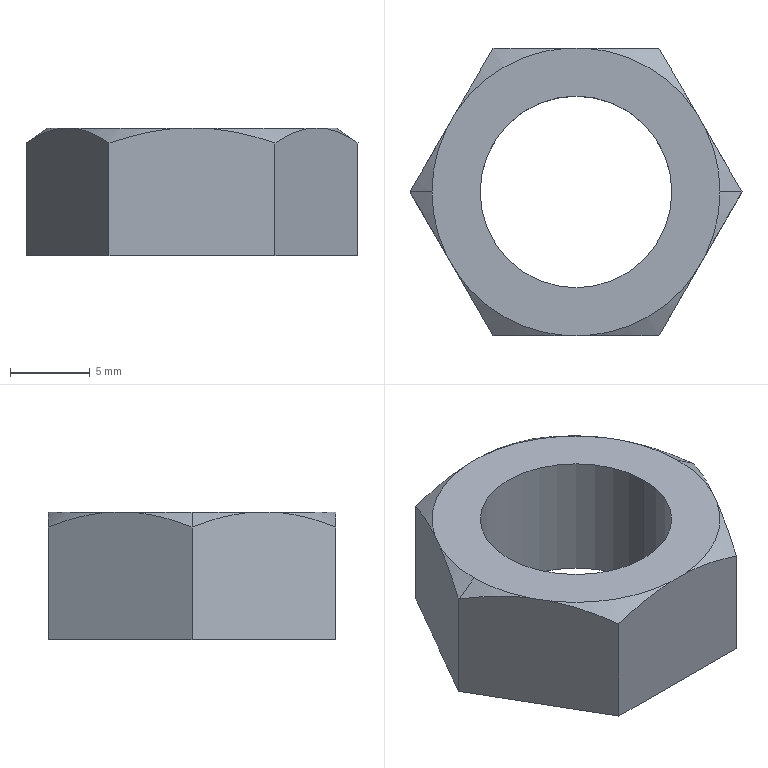Part | NX | features solid 2 | 1 solid | 18 faces | box 20.785 x 18 x 8 mm | volume 1333 mm3 | cone 8 | plane 8 | cylinder 2 | commonest cylinder face diameters 12 x2
STEP:
#1=CARTESIAN_POINT('',(-251.91,-30.511,-1188.5));
#2=VERTEX_POINT('',#1);
#3=CARTESIAN_POINT('',(-249.608,-34.5,-1189.432));
#4=VERTEX_POINT('',#3);
#5=CARTESIAN_POINT('',(-251.91,-30.511,-1188.5));
#6=CARTESIAN_POINT('',(-251.119,-31.883,-1188.57));
#7=CARTESIAN_POINT('',(-250.355,-33.205,-1188.925));
#8=CARTESIAN_POINT('',(-249.608,-34.5,-1189.432));
#9=B_SPLINE_CURVE_WITH_KNOTS('',3,(#5,#6,#7,#8),.UNSPECIFIED.,.F.,.F.,(4,4),(0.,0.004699),.UNSPECIFIED.);
#10=EDGE_CURVE('',#2,#4,#9,.T.);
#11=ORIENTED_EDGE('',*,*,#10,.F.);
#12=CARTESIAN_POINT('',(-250.981,-34.5,-1188.5));
#13=VERTEX_POINT('',#12);
#14=CARTESIAN_POINT('',(-260.,-34.5,-1188.5));
#15=DIRECTION('',(0.,0.,-1.));
#16=DIRECTION('',(0.8969,0.4422,0.));
#17=AXIS2_PLACEMENT_3D('',#14,#15,#16);
#18=CIRCLE('',#17,9.019);
#19=EDGE_CURVE('',#2,#13,#18,.T.);
#20=ORIENTED_EDGE('',*,*,#19,.T.);
#21=CARTESIAN_POINT('',(-249.608,-34.5,-1189.432));
#22=DIRECTION('',(-0.8273,0.,0.5618));
#23=VECTOR('',#22,1000.);
#24=LINE('',#21,#23);
#25=EDGE_CURVE('',#4,#13,#24,.T.);
#26=ORIENTED_EDGE('',*,*,#25,.F.);
#27=EDGE_LOOP('',(#11,#20,#26));
#28=FACE_BOUND('',#27,.T.);
#29=CARTESIAN_POINT('',(-260.,-34.5,-1188.966));
#30=DIRECTION('',(0.,0.,-1.));
#31=DIRECTION('',(1.,0.,0.));
#32=AXIS2_PLACEMENT_3D('',#29,#30,#31);
#33=CONICAL_SURFACE('',#32,9.706,0.9742);
#34=ADVANCED_FACE('',(#28),#33,.T.);
#35=CARTESIAN_POINT('',(-251.91,-38.489,-1188.5));
#36=VERTEX_POINT('',#35);
#37=CARTESIAN_POINT('',(-260.,-34.5,-1188.5));
#38=DIRECTION('',(0.,0.,-1.));
#39=DIRECTION('',(1.,0.,0.));
#40=AXIS2_PLACEMENT_3D('',#37,#38,#39);
#41=CIRCLE('',#40,9.019);
#42=EDGE_CURVE('',#13,#36,#41,.T.);
#43=ORIENTED_EDGE('',*,*,#42,.T.);
#44=CARTESIAN_POINT('',(-251.91,-38.489,-1188.5));
#45=CARTESIAN_POINT('',(-251.816,-38.324,-1188.508));
#46=CARTESIAN_POINT('',(-251.626,-37.996,-1188.533));
#47=CARTESIAN_POINT('',(-251.344,-37.507,-1188.594));
#48=CARTESIAN_POINT('',(-251.062,-37.018,-1188.678));
#49=CARTESIAN_POINT('',(-250.779,-36.528,-1188.783));
#50=CARTESIAN_POINT('',(-250.494,-36.036,-1188.911));
#51=CARTESIAN_POINT('',(-250.207,-35.537,-1189.06));
#52=CARTESIAN_POINT('',(-249.913,-35.028,-1189.231));
#53=CARTESIAN_POINT('',(-249.71,-34.678,-1189.363));
#54=CARTESIAN_POINT('',(-249.608,-34.5,-1189.432));
#55=B_SPLINE_CURVE_WITH_KNOTS('',3,(#44,#45,#46,#47,#48,#49,#50,#51,#52,#53,#54),.UNSPECIFIED.,.F.,.F.,(4,1,1,1,1,1,1,1,4),(0.,0.125,0.25,0.375,0.5,0.625,0.75,0.875,1.),.QUASI_UNIFORM_KNOTS.);
#56=EDGE_CURVE('',#36,#4,#55,.T.);
#57=ORIENTED_EDGE('',*,*,#56,.T.);
#58=ORIENTED_EDGE('',*,*,#25,.T.);
#59=EDGE_LOOP('',(#43,#57,#58));
#60=FACE_BOUND('',#59,.T.);
#61=CARTESIAN_POINT('',(-260.,-34.5,-1188.966));
#62=DIRECTION('',(0.,0.,-1.));
#63=DIRECTION('',(1.,0.,0.));
#64=AXIS2_PLACEMENT_3D('',#61,#62,#63);
#65=CONICAL_SURFACE('',#64,9.706,0.9742);
#66=ADVANCED_FACE('',(#60),#65,.T.);
#67=CARTESIAN_POINT('',(-254.804,-43.5,-1196.5));
#68=VERTEX_POINT('',#67);
#69=CARTESIAN_POINT('',(-249.608,-34.5,-1196.5));
#70=VERTEX_POINT('',#69);
#71=CARTESIAN_POINT('',(-254.804,-43.5,-1196.5));
#72=DIRECTION('',(0.5,0.866,0.));
#73=VECTOR('',#72,1000.);
#74=LINE('',#71,#73);
#75=EDGE_CURVE('',#68,#70,#74,.T.);
#76=ORIENTED_EDGE('',*,*,#75,.T.);
#77=CARTESIAN_POINT('',(-249.608,-34.5,-1196.5));
#78=DIRECTION('',(0.,0.,1.));
#79=VECTOR('',#78,1000.);
#80=LINE('',#77,#79);
#81=EDGE_CURVE('',#70,#4,#80,.T.);
#82=ORIENTED_EDGE('',*,*,#81,.T.);
#83=ORIENTED_EDGE('',*,*,#56,.F.);
#84=CARTESIAN_POINT('',(-252.501,-39.511,-1188.5));
#85=VERTEX_POINT('',#84);
#86=CARTESIAN_POINT('',(-251.91,-38.489,-1188.5));
#87=DIRECTION('',(-0.5,-0.866,0.000000195));
#88=VECTOR('',#87,1000.);
#89=LINE('',#86,#88);
#90=EDGE_CURVE('',#36,#85,#89,.T.);
#91=ORIENTED_EDGE('',*,*,#90,.T.);
#92=CARTESIAN_POINT('',(-254.804,-43.5,-1189.432));
#93=VERTEX_POINT('',#92);
#94=CARTESIAN_POINT('',(-252.501,-39.511,-1188.5));
#95=CARTESIAN_POINT('',(-253.293,-40.883,-1188.57));
#96=CARTESIAN_POINT('',(-254.056,-42.205,-1188.925));
#97=CARTESIAN_POINT('',(-254.804,-43.5,-1189.432));
#98=B_SPLINE_CURVE_WITH_KNOTS('',3,(#94,#95,#96,#97),.UNSPECIFIED.,.F.,.F.,(4,4),(0.,0.004699),.UNSPECIFIED.);
#99=EDGE_CURVE('',#85,#93,#98,.T.);
#100=ORIENTED_EDGE('',*,*,#99,.T.);
#101=CARTESIAN_POINT('',(-254.804,-43.5,-1196.5));
#102=DIRECTION('',(0.,0.,1.));
#103=VECTOR('',#102,1000.);
#104=LINE('',#101,#103);
#105=EDGE_CURVE('',#68,#93,#104,.T.);
#106=ORIENTED_EDGE('',*,*,#105,.F.);
#107=EDGE_LOOP('',(#76,#82,#83,#91,#100,#106));
#108=FACE_BOUND('',#107,.T.);
#109=CARTESIAN_POINT('',(-254.804,-43.5,-1196.5));
#110=DIRECTION('',(0.866,-0.5,0.));
#111=DIRECTION('',(-0.5,-0.866,0.));
#112=AXIS2_PLACEMENT_3D('',#109,#110,#111);
#113=PLANE('',#112);
#114=ADVANCED_FACE('',(#108),#113,.T.);
#115=CARTESIAN_POINT('',(-265.196,-43.5,-1196.5));
#116=VERTEX_POINT('',#115);
#117=CARTESIAN_POINT('',(-265.196,-43.5,-1196.5));
#118=DIRECTION('',(1.,0.,0.));
#119=VECTOR('',#118,1000.);
#120=LINE('',#117,#119);
#121=EDGE_CURVE('',#116,#68,#120,.T.);
#122=ORIENTED_EDGE('',*,*,#121,.T.);
#123=ORIENTED_EDGE('',*,*,#105,.T.);
#124=CARTESIAN_POINT('',(-259.409,-43.5,-1188.5));
#125=VERTEX_POINT('',#124);
#126=CARTESIAN_POINT('',(-259.409,-43.5,-1188.5));
#127=CARTESIAN_POINT('',(-259.22,-43.5,-1188.508));
#128=CARTESIAN_POINT('',(-258.841,-43.5,-1188.533));
#129=CARTESIAN_POINT('',(-258.276,-43.5,-1188.594));
#130=CARTESIAN_POINT('',(-257.712,-43.5,-1188.678));
#131=CARTESIAN_POINT('',(-257.146,-43.5,-1188.783));
#132=CARTESIAN_POINT('',(-256.577,-43.5,-1188.911));
#133=CARTESIAN_POINT('',(-256.002,-43.5,-1189.06));
#134=CARTESIAN_POINT('',(-255.414,-43.5,-1189.231));
#135=CARTESIAN_POINT('',(-255.009,-43.5,-1189.363));
#136=CARTESIAN_POINT('',(-254.804,-43.5,-1189.432));
#137=B_SPLINE_CURVE_WITH_KNOTS('',3,(#126,#127,#128,#129,#130,#131,#132,#133,#134,#135,#136),.UNSPECIFIED.,.F.,.F.,(4,1,1,1,1,1,1,1,4),(0.,0.125,0.25,0.375,0.5,0.625,0.75,0.875,1.),.QUASI_UNIFORM_KNOTS.);
#138=EDGE_CURVE('',#125,#93,#137,.T.);
#139=ORIENTED_EDGE('',*,*,#138,.F.);
#140=CARTESIAN_POINT('',(-260.591,-43.5,-1188.5));
#141=VERTEX_POINT('',#140);
#142=CARTESIAN_POINT('',(-259.409,-43.5,-1188.5));
#143=DIRECTION('',(-1.,-0.000000007,0.));
#144=VECTOR('',#143,1000.);
#145=LINE('',#142,#144);
#146=EDGE_CURVE('',#125,#141,#145,.T.);
#147=ORIENTED_EDGE('',*,*,#146,.T.);
#148=CARTESIAN_POINT('',(-265.196,-43.5,-1189.432));
#149=VERTEX_POINT('',#148);
#150=CARTESIAN_POINT('',(-260.591,-43.5,-1188.5));
#151=CARTESIAN_POINT('',(-262.174,-43.5,-1188.57));
#152=CARTESIAN_POINT('',(-263.701,-43.5,-1188.925));
#153=CARTESIAN_POINT('',(-265.196,-43.5,-1189.432));
#154=B_SPLINE_CURVE_WITH_KNOTS('',3,(#150,#151,#152,#153),.UNSPECIFIED.,.F.,.F.,(4,4),(0.,0.004699),.UNSPECIFIED.);
#155=EDGE_CURVE('',#141,#149,#154,.T.);
#156=ORIENTED_EDGE('',*,*,#155,.T.);
#157=CARTESIAN_POINT('',(-265.196,-43.5,-1196.5));
#158=DIRECTION('',(0.,0.,1.));
#159=VECTOR('',#158,1000.);
#160=LINE('',#157,#159);
#161=EDGE_CURVE('',#116,#149,#160,.T.);
#162=ORIENTED_EDGE('',*,*,#161,.F.);
#163=EDGE_LOOP('',(#122,#123,#139,#147,#156,#162));
#164=FACE_BOUND('',#163,.T.);
#165=CARTESIAN_POINT('',(-265.196,-43.5,-1196.5));
#166=DIRECTION('',(0.,-1.,0.));
#167=DIRECTION('',(-1.,0.,0.));
#168=AXIS2_PLACEMENT_3D('',#165,#166,#167);
#169=PLANE('',#168);
#170=ADVANCED_FACE('',(#164),#169,.T.);
#171=CARTESIAN_POINT('',(-270.392,-34.5,-1196.5));
#172=VERTEX_POINT('',#171);
#173=CARTESIAN_POINT('',(-270.392,-34.5,-1196.5));
#174=DIRECTION('',(0.5,-0.866,0.));
#175=VECTOR('',#174,1000.);
#176=LINE('',#173,#175);
#177=EDGE_CURVE('',#172,#116,#176,.T.);
#178=ORIENTED_EDGE('',*,*,#177,.T.);
#179=ORIENTED_EDGE('',*,*,#161,.T.);
#180=CARTESIAN_POINT('',(-267.499,-39.511,-1188.5));
#181=VERTEX_POINT('',#180);
#182=CARTESIAN_POINT('',(-267.499,-39.511,-1188.5));
#183=CARTESIAN_POINT('',(-267.404,-39.676,-1188.508));
#184=CARTESIAN_POINT('',(-267.215,-40.004,-1188.533));
#185=CARTESIAN_POINT('',(-266.932,-40.493,-1188.594));
#186=CARTESIAN_POINT('',(-266.65,-40.982,-1188.678));
#187=CARTESIAN_POINT('',(-266.367,-41.472,-1188.783));
#188=CARTESIAN_POINT('',(-266.083,-41.964,-1188.911));
#189=CARTESIAN_POINT('',(-265.795,-42.463,-1189.06));
#190=CARTESIAN_POINT('',(-265.501,-42.972,-1189.231));
#191=CARTESIAN_POINT('',(-265.299,-43.322,-1189.363));
#192=CARTESIAN_POINT('',(-265.196,-43.5,-1189.432));
#193=B_SPLINE_CURVE_WITH_KNOTS('',3,(#182,#183,#184,#185,#186,#187,#188,#189,#190,#191,#192),.UNSPECIFIED.,.F.,.F.,(4,1,1,1,1,1,1,1,4),(0.,0.125,0.25,0.375,0.5,0.625,0.75,0.875,1.),.QUASI_UNIFORM_KNOTS.);
#194=EDGE_CURVE('',#181,#149,#193,.T.);
#195=ORIENTED_EDGE('',*,*,#194,.F.);
#196=CARTESIAN_POINT('',(-268.09,-38.489,-1188.5));
#197=VERTEX_POINT('',#196);
#198=CARTESIAN_POINT('',(-267.499,-39.511,-1188.5));
#199=DIRECTION('',(-0.5,0.866,-0.000000195));
#200=VECTOR('',#199,1000.);
#201=LINE('',#198,#200);
#202=EDGE_CURVE('',#181,#197,#201,.T.);
#203=ORIENTED_EDGE('',*,*,#202,.T.);
#204=CARTESIAN_POINT('',(-270.392,-34.5,-1189.432));
#205=VERTEX_POINT('',#204);
#206=CARTESIAN_POINT('',(-268.09,-38.489,-1188.5));
#207=CARTESIAN_POINT('',(-268.881,-37.117,-1188.57));
#208=CARTESIAN_POINT('',(-269.645,-35.795,-1188.925));
#209=CARTESIAN_POINT('',(-270.392,-34.5,-1189.432));
#210=B_SPLINE_CURVE_WITH_KNOTS('',3,(#206,#207,#208,#209),.UNSPECIFIED.,.F.,.F.,(4,4),(0.,0.004699),.UNSPECIFIED.);
#211=EDGE_CURVE('',#197,#205,#210,.T.);
#212=ORIENTED_EDGE('',*,*,#211,.T.);
#213=CARTESIAN_POINT('',(-270.392,-34.5,-1196.5));
#214=DIRECTION('',(0.,0.,1.));
#215=VECTOR('',#214,1000.);
#216=LINE('',#213,#215);
#217=EDGE_CURVE('',#172,#205,#216,.T.);
#218=ORIENTED_EDGE('',*,*,#217,.F.);
#219=EDGE_LOOP('',(#178,#179,#195,#203,#212,#218));
#220=FACE_BOUND('',#219,.T.);
#221=CARTESIAN_POINT('',(-270.392,-34.5,-1196.5));
#222=DIRECTION('',(-0.866,-0.5,0.));
#223=DIRECTION('',(-0.5,0.866,0.));
#224=AXIS2_PLACEMENT_3D('',#221,#222,#223);
#225=PLANE('',#224);
#226=ADVANCED_FACE('',(#220),#225,.T.);
#227=CARTESIAN_POINT('',(-265.196,-25.5,-1196.5));
#228=VERTEX_POINT('',#227);
#229=CARTESIAN_POINT('',(-265.196,-25.5,-1196.5));
#230=DIRECTION('',(-0.5,-0.866,0.));
#231=VECTOR('',#230,1000.);
#232=LINE('',#229,#231);
#233=EDGE_CURVE('',#228,#172,#232,.T.);
#234=ORIENTED_EDGE('',*,*,#233,.T.);
#235=ORIENTED_EDGE('',*,*,#217,.T.);
#236=CARTESIAN_POINT('',(-268.09,-30.511,-1188.5));
#237=VERTEX_POINT('',#236);
#238=CARTESIAN_POINT('',(-268.09,-30.511,-1188.5));
#239=CARTESIAN_POINT('',(-268.184,-30.676,-1188.508));
#240=CARTESIAN_POINT('',(-268.374,-31.004,-1188.533));
#241=CARTESIAN_POINT('',(-268.656,-31.493,-1188.594));
#242=CARTESIAN_POINT('',(-268.938,-31.982,-1188.678));
#243=CARTESIAN_POINT('',(-269.221,-32.472,-1188.783));
#244=CARTESIAN_POINT('',(-269.506,-32.964,-1188.911));
#245=CARTESIAN_POINT('',(-269.793,-33.463,-1189.06));
#246=CARTESIAN_POINT('',(-270.087,-33.972,-1189.231));
#247=CARTESIAN_POINT('',(-270.29,-34.322,-1189.363));
#248=CARTESIAN_POINT('',(-270.392,-34.5,-1189.432));
#249=B_SPLINE_CURVE_WITH_KNOTS('',3,(#238,#239,#240,#241,#242,#243,#244,#245,#246,#247,#248),.UNSPECIFIED.,.F.,.F.,(4,1,1,1,1,1,1,1,4),(0.,0.125,0.25,0.375,0.5,0.625,0.75,0.875,1.),.QUASI_UNIFORM_KNOTS.);
#250=EDGE_CURVE('',#237,#205,#249,.T.);
#251=ORIENTED_EDGE('',*,*,#250,.F.);
#252=CARTESIAN_POINT('',(-267.499,-29.489,-1188.5));
#253=VERTEX_POINT('',#252);
#254=CARTESIAN_POINT('',(-268.09,-30.511,-1188.5));
#255=DIRECTION('',(0.5,0.866,0.000000195));
#256=VECTOR('',#255,1000.);
#257=LINE('',#254,#256);
#258=EDGE_CURVE('',#237,#253,#257,.T.);
#259=ORIENTED_EDGE('',*,*,#258,.T.);
#260=CARTESIAN_POINT('',(-265.196,-25.5,-1189.432));
#261=VERTEX_POINT('',#260);
#262=CARTESIAN_POINT('',(-267.499,-29.489,-1188.5));
#263=CARTESIAN_POINT('',(-266.707,-28.117,-1188.57));
#264=CARTESIAN_POINT('',(-265.944,-26.795,-1188.925));
#265=CARTESIAN_POINT('',(-265.196,-25.5,-1189.432));
#266=B_SPLINE_CURVE_WITH_KNOTS('',3,(#262,#263,#264,#265),.UNSPECIFIED.,.F.,.F.,(4,4),(0.,0.004699),.UNSPECIFIED.);
#267=EDGE_CURVE('',#253,#261,#266,.T.);
#268=ORIENTED_EDGE('',*,*,#267,.T.);
#269=CARTESIAN_POINT('',(-265.196,-25.5,-1196.5));
#270=DIRECTION('',(0.,0.,1.));
#271=VECTOR('',#270,1000.);
#272=LINE('',#269,#271);
#273=EDGE_CURVE('',#228,#261,#272,.T.);
#274=ORIENTED_EDGE('',*,*,#273,.F.);
#275=EDGE_LOOP('',(#234,#235,#251,#259,#268,#274));
#276=FACE_BOUND('',#275,.T.);
#277=CARTESIAN_POINT('',(-265.196,-25.5,-1196.5));
#278=DIRECTION('',(-0.866,0.5,0.));
#279=DIRECTION('',(0.5,0.866,0.));
#280=AXIS2_PLACEMENT_3D('',#277,#278,#279);
#281=PLANE('',#280);
#282=ADVANCED_FACE('',(#276),#281,.T.);
#283=CARTESIAN_POINT('',(-254.804,-25.5,-1196.5));
#284=VERTEX_POINT('',#283);
#285=CARTESIAN_POINT('',(-254.804,-25.5,-1196.5));
#286=DIRECTION('',(-1.,0.,0.));
#287=VECTOR('',#286,1000.);
#288=LINE('',#285,#287);
#289=EDGE_CURVE('',#284,#228,#288,.T.);
#290=ORIENTED_EDGE('',*,*,#289,.T.);
#291=ORIENTED_EDGE('',*,*,#273,.T.);
#292=CARTESIAN_POINT('',(-260.591,-25.5,-1188.5));
#293=VERTEX_POINT('',#292);
#294=CARTESIAN_POINT('',(-260.591,-25.5,-1188.5));
#295=CARTESIAN_POINT('',(-260.78,-25.5,-1188.508));
#296=CARTESIAN_POINT('',(-261.159,-25.5,-1188.533));
#297=CARTESIAN_POINT('',(-261.724,-25.5,-1188.594));
#298=CARTESIAN_POINT('',(-262.288,-25.5,-1188.678));
#299=CARTESIAN_POINT('',(-262.854,-25.5,-1188.783));
#300=CARTESIAN_POINT('',(-263.423,-25.5,-1188.911));
#301=CARTESIAN_POINT('',(-263.998,-25.5,-1189.06));
#302=CARTESIAN_POINT('',(-264.586,-25.5,-1189.231));
#303=CARTESIAN_POINT('',(-264.991,-25.5,-1189.363));
#304=CARTESIAN_POINT('',(-265.196,-25.5,-1189.432));
#305=B_SPLINE_CURVE_WITH_KNOTS('',3,(#294,#295,#296,#297,#298,#299,#300,#301,#302,#303,#304),.UNSPECIFIED.,.F.,.F.,(4,1,1,1,1,1,1,1,4),(0.,0.125,0.25,0.375,0.5,0.625,0.75,0.875,1.),.QUASI_UNIFORM_KNOTS.);
#306=EDGE_CURVE('',#293,#261,#305,.T.);
#307=ORIENTED_EDGE('',*,*,#306,.F.);
#308=CARTESIAN_POINT('',(-259.409,-25.5,-1188.5));
#309=VERTEX_POINT('',#308);
#310=CARTESIAN_POINT('',(-260.591,-25.5,-1188.5));
#311=DIRECTION('',(1.,0.000000007,0.));
#312=VECTOR('',#311,1000.);
#313=LINE('',#310,#312);
#314=EDGE_CURVE('',#293,#309,#313,.T.);
#315=ORIENTED_EDGE('',*,*,#314,.T.);
#316=CARTESIAN_POINT('',(-254.804,-25.5,-1189.432));
#317=VERTEX_POINT('',#316);
#318=CARTESIAN_POINT('',(-259.409,-25.5,-1188.5));
#319=CARTESIAN_POINT('',(-257.826,-25.5,-1188.57));
#320=CARTESIAN_POINT('',(-256.299,-25.5,-1188.925));
#321=CARTESIAN_POINT('',(-254.804,-25.5,-1189.432));
#322=B_SPLINE_CURVE_WITH_KNOTS('',3,(#318,#319,#320,#321),.UNSPECIFIED.,.F.,.F.,(4,4),(0.,0.004699),.UNSPECIFIED.);
#323=EDGE_CURVE('',#309,#317,#322,.T.);
#324=ORIENTED_EDGE('',*,*,#323,.T.);
#325=CARTESIAN_POINT('',(-254.804,-25.5,-1189.432));
#326=DIRECTION('',(0.,0.,-1.));
#327=VECTOR('',#326,1000.);
#328=LINE('',#325,#327);
#329=EDGE_CURVE('',#317,#284,#328,.T.);
#330=ORIENTED_EDGE('',*,*,#329,.T.);
#331=EDGE_LOOP('',(#290,#291,#307,#315,#324,#330));
#332=FACE_BOUND('',#331,.T.);
#333=CARTESIAN_POINT('',(-254.804,-25.5,-1196.5));
#334=DIRECTION('',(0.,1.,0.));
#335=DIRECTION('',(1.,0.,0.));
#336=AXIS2_PLACEMENT_3D('',#333,#334,#335);
#337=PLANE('',#336);
#338=ADVANCED_FACE('',(#332),#337,.T.);
#339=CARTESIAN_POINT('',(-249.608,-34.5,-1196.5));
#340=DIRECTION('',(-0.5,0.866,0.));
#341=VECTOR('',#340,1000.);
#342=LINE('',#339,#341);
#343=EDGE_CURVE('',#70,#284,#342,.T.);
#344=ORIENTED_EDGE('',*,*,#343,.T.);
#345=ORIENTED_EDGE('',*,*,#329,.F.);
#346=CARTESIAN_POINT('',(-252.501,-29.489,-1188.5));
#347=VERTEX_POINT('',#346);
#348=CARTESIAN_POINT('',(-252.501,-29.489,-1188.5));
#349=CARTESIAN_POINT('',(-252.596,-29.324,-1188.508));
#350=CARTESIAN_POINT('',(-252.785,-28.996,-1188.533));
#351=CARTESIAN_POINT('',(-253.068,-28.507,-1188.594));
#352=CARTESIAN_POINT('',(-253.35,-28.018,-1188.678));
#353=CARTESIAN_POINT('',(-253.633,-27.528,-1188.783));
#354=CARTESIAN_POINT('',(-253.917,-27.036,-1188.911));
#355=CARTESIAN_POINT('',(-254.205,-26.537,-1189.06));
#356=CARTESIAN_POINT('',(-254.499,-26.028,-1189.231));
#357=CARTESIAN_POINT('',(-254.701,-25.678,-1189.363));
#358=CARTESIAN_POINT('',(-254.804,-25.5,-1189.432));
#359=B_SPLINE_CURVE_WITH_KNOTS('',3,(#348,#349,#350,#351,#352,#353,#354,#355,#356,#357,#358),.UNSPECIFIED.,.F.,.F.,(4,1,1,1,1,1,1,1,4),(0.,0.125,0.25,0.375,0.5,0.625,0.75,0.875,1.),.QUASI_UNIFORM_KNOTS.);
#360=EDGE_CURVE('',#347,#317,#359,.T.);
#361=ORIENTED_EDGE('',*,*,#360,.F.);
#362=CARTESIAN_POINT('',(-252.501,-29.489,-1188.5));
#363=DIRECTION('',(0.5,-0.866,-0.000000195));
#364=VECTOR('',#363,1000.);
#365=LINE('',#362,#364);
#366=EDGE_CURVE('',#347,#2,#365,.T.);
#367=ORIENTED_EDGE('',*,*,#366,.T.);
#368=ORIENTED_EDGE('',*,*,#10,.T.);
#369=ORIENTED_EDGE('',*,*,#81,.F.);
#370=EDGE_LOOP('',(#344,#345,#361,#367,#368,#369));
#371=FACE_BOUND('',#370,.T.);
#372=CARTESIAN_POINT('',(-249.608,-34.5,-1196.5));
#373=DIRECTION('',(0.866,0.5,0.));
#374=DIRECTION('',(0.5,-0.866,0.));
#375=AXIS2_PLACEMENT_3D('',#372,#373,#374);
#376=PLANE('',#375);
#377=ADVANCED_FACE('',(#371),#376,.T.);
#378=CARTESIAN_POINT('',(-260.,-34.5,-1188.5));
#379=DIRECTION('',(0.,0.,-1.));
#380=DIRECTION('',(0.06548,0.9979,0.));
#381=AXIS2_PLACEMENT_3D('',#378,#379,#380);
#382=CIRCLE('',#381,9.019);
#383=EDGE_CURVE('',#309,#347,#382,.T.);
#384=ORIENTED_EDGE('',*,*,#383,.F.);
#385=ORIENTED_EDGE('',*,*,#314,.F.);
#386=CARTESIAN_POINT('',(-260.,-34.5,-1188.5));
#387=DIRECTION('',(0.,0.,-1.));
#388=DIRECTION('',(-0.8314,0.5556,0.));
#389=AXIS2_PLACEMENT_3D('',#386,#387,#388);
#390=CIRCLE('',#389,9.019);
#391=EDGE_CURVE('',#253,#293,#390,.T.);
#392=ORIENTED_EDGE('',*,*,#391,.F.);
#393=ORIENTED_EDGE('',*,*,#258,.F.);
#394=CARTESIAN_POINT('',(-269.019,-34.5,-1188.5));
#395=VERTEX_POINT('',#394);
#396=CARTESIAN_POINT('',(-260.,-34.5,-1188.5));
#397=DIRECTION('',(0.,0.,-1.));
#398=DIRECTION('',(-1.,0.,0.));
#399=AXIS2_PLACEMENT_3D('',#396,#397,#398);
#400=CIRCLE('',#399,9.019);
#401=EDGE_CURVE('',#395,#237,#400,.T.);
#402=ORIENTED_EDGE('',*,*,#401,.F.);
#403=CARTESIAN_POINT('',(-260.,-34.5,-1188.5));
#404=DIRECTION('',(0.,0.,-1.));
#405=DIRECTION('',(-0.8969,-0.4422,0.));
#406=AXIS2_PLACEMENT_3D('',#403,#404,#405);
#407=CIRCLE('',#406,9.019);
#408=EDGE_CURVE('',#197,#395,#407,.T.);
#409=ORIENTED_EDGE('',*,*,#408,.F.);
#410=ORIENTED_EDGE('',*,*,#202,.F.);
#411=CARTESIAN_POINT('',(-260.,-34.5,-1188.5));
#412=DIRECTION('',(0.,0.,-1.));
#413=DIRECTION('',(-0.06548,-0.9979,0.));
#414=AXIS2_PLACEMENT_3D('',#411,#412,#413);
#415=CIRCLE('',#414,9.019);
#416=EDGE_CURVE('',#141,#181,#415,.T.);
#417=ORIENTED_EDGE('',*,*,#416,.F.);
#418=ORIENTED_EDGE('',*,*,#146,.F.);
#419=CARTESIAN_POINT('',(-260.,-34.5,-1188.5));
#420=DIRECTION('',(0.,0.,-1.));
#421=DIRECTION('',(0.8314,-0.5556,0.));
#422=AXIS2_PLACEMENT_3D('',#419,#420,#421);
#423=CIRCLE('',#422,9.019);
#424=EDGE_CURVE('',#85,#125,#423,.T.);
#425=ORIENTED_EDGE('',*,*,#424,.F.);
#426=ORIENTED_EDGE('',*,*,#90,.F.);
#427=ORIENTED_EDGE('',*,*,#42,.F.);
#428=ORIENTED_EDGE('',*,*,#19,.F.);
#429=ORIENTED_EDGE('',*,*,#366,.F.);
#430=EDGE_LOOP('',(#384,#385,#392,#393,#402,#409,#410,#417,#418,#425,#426,#427,#428,#429));
#431=FACE_BOUND('',#430,.T.);
#432=CARTESIAN_POINT('',(-266.,-34.5,-1188.5));
#433=VERTEX_POINT('',#432);
#434=CARTESIAN_POINT('',(-254.,-34.5,-1188.5));
#435=VERTEX_POINT('',#434);
#436=CARTESIAN_POINT('',(-260.,-34.5,-1188.5));
#437=DIRECTION('',(0.,0.,1.));
#438=DIRECTION('',(-1.,0.,0.));
#439=AXIS2_PLACEMENT_3D('',#436,#437,#438);
#440=CIRCLE('',#439,6.);
#441=EDGE_CURVE('',#433,#435,#440,.T.);
#442=ORIENTED_EDGE('',*,*,#441,.F.);
#443=CARTESIAN_POINT('',(-260.,-34.5,-1188.5));
#444=DIRECTION('',(0.,0.,1.));
#445=DIRECTION('',(1.,0.,0.));
#446=AXIS2_PLACEMENT_3D('',#443,#444,#445);
#447=CIRCLE('',#446,6.);
#448=EDGE_CURVE('',#435,#433,#447,.T.);
#449=ORIENTED_EDGE('',*,*,#448,.F.);
#450=EDGE_LOOP('',(#442,#449));
#451=FACE_BOUND('',#450,.T.);
#452=CARTESIAN_POINT('',(-260.,-34.5,-1188.5));
#453=DIRECTION('',(0.,0.,1.));
#454=DIRECTION('',(1.,0.,0.));
#455=AXIS2_PLACEMENT_3D('',#452,#453,#454);
#456=PLANE('',#455);
#457=ADVANCED_FACE('',(#431,#451),#456,.T.);
#458=ORIENTED_EDGE('',*,*,#138,.T.);
#459=ORIENTED_EDGE('',*,*,#99,.F.);
#460=ORIENTED_EDGE('',*,*,#424,.T.);
#461=EDGE_LOOP('',(#458,#459,#460));
#462=FACE_BOUND('',#461,.T.);
#463=CARTESIAN_POINT('',(-260.,-34.5,-1188.966));
#464=DIRECTION('',(0.,0.,-1.));
#465=DIRECTION('',(1.,0.,0.));
#466=AXIS2_PLACEMENT_3D('',#463,#464,#465);
#467=CONICAL_SURFACE('',#466,9.706,0.9742);
#468=ADVANCED_FACE('',(#462),#467,.T.);
#469=ORIENTED_EDGE('',*,*,#194,.T.);
#470=ORIENTED_EDGE('',*,*,#155,.F.);
#471=ORIENTED_EDGE('',*,*,#416,.T.);
#472=EDGE_LOOP('',(#469,#470,#471));
#473=FACE_BOUND('',#472,.T.);
#474=CARTESIAN_POINT('',(-260.,-34.5,-1188.966));
#475=DIRECTION('',(0.,0.,-1.));
#476=DIRECTION('',(1.,0.,0.));
#477=AXIS2_PLACEMENT_3D('',#474,#475,#476);
#478=CONICAL_SURFACE('',#477,9.706,0.9742);
#479=ADVANCED_FACE('',(#473),#478,.T.);
#480=ORIENTED_EDGE('',*,*,#211,.F.);
#481=ORIENTED_EDGE('',*,*,#408,.T.);
#482=CARTESIAN_POINT('',(-269.019,-34.5,-1188.5));
#483=DIRECTION('',(-0.8273,0.,-0.5618));
#484=VECTOR('',#483,1000.);
#485=LINE('',#482,#484);
#486=EDGE_CURVE('',#395,#205,#485,.T.);
#487=ORIENTED_EDGE('',*,*,#486,.T.);
#488=EDGE_LOOP('',(#480,#481,#487));
#489=FACE_BOUND('',#488,.T.);
#490=CARTESIAN_POINT('',(-260.,-34.5,-1188.966));
#491=DIRECTION('',(0.,0.,-1.));
#492=DIRECTION('',(1.,0.,0.));
#493=AXIS2_PLACEMENT_3D('',#490,#491,#492);
#494=CONICAL_SURFACE('',#493,9.706,0.9742);
#495=ADVANCED_FACE('',(#489),#494,.T.);
#496=ORIENTED_EDGE('',*,*,#401,.T.);
#497=ORIENTED_EDGE('',*,*,#250,.T.);
#498=ORIENTED_EDGE('',*,*,#486,.F.);
#499=EDGE_LOOP('',(#496,#497,#498));
#500=FACE_BOUND('',#499,.T.);
#501=CARTESIAN_POINT('',(-260.,-34.5,-1188.966));
#502=DIRECTION('',(0.,0.,-1.));
#503=DIRECTION('',(1.,0.,0.));
#504=AXIS2_PLACEMENT_3D('',#501,#502,#503);
#505=CONICAL_SURFACE('',#504,9.706,0.9742);
#506=ADVANCED_FACE('',(#500),#505,.T.);
#507=ORIENTED_EDGE('',*,*,#306,.T.);
#508=ORIENTED_EDGE('',*,*,#267,.F.);
#509=ORIENTED_EDGE('',*,*,#391,.T.);
#510=EDGE_LOOP('',(#507,#508,#509));
#511=FACE_BOUND('',#510,.T.);
#512=CARTESIAN_POINT('',(-260.,-34.5,-1188.966));
#513=DIRECTION('',(0.,0.,-1.));
#514=DIRECTION('',(1.,0.,0.));
#515=AXIS2_PLACEMENT_3D('',#512,#513,#514);
#516=CONICAL_SURFACE('',#515,9.706,0.9742);
#517=ADVANCED_FACE('',(#511),#516,.T.);
#518=ORIENTED_EDGE('',*,*,#360,.T.);
#519=ORIENTED_EDGE('',*,*,#323,.F.);
#520=ORIENTED_EDGE('',*,*,#383,.T.);
#521=EDGE_LOOP('',(#518,#519,#520));
#522=FACE_BOUND('',#521,.T.);
#523=CARTESIAN_POINT('',(-260.,-34.5,-1188.966));
#524=DIRECTION('',(0.,0.,-1.));
#525=DIRECTION('',(1.,0.,0.));
#526=AXIS2_PLACEMENT_3D('',#523,#524,#525);
#527=CONICAL_SURFACE('',#526,9.706,0.9742);
#528=ADVANCED_FACE('',(#522),#527,.T.);
#529=CARTESIAN_POINT('',(-266.,-34.5,-1196.5));
#530=VERTEX_POINT('',#529);
#531=CARTESIAN_POINT('',(-254.,-34.5,-1196.5));
#532=VERTEX_POINT('',#531);
#533=CARTESIAN_POINT('',(-260.,-34.5,-1196.5));
#534=DIRECTION('',(0.,0.,-1.));
#535=DIRECTION('',(-1.,0.,0.));
#536=AXIS2_PLACEMENT_3D('',#533,#534,#535);
#537=CIRCLE('',#536,6.);
#538=EDGE_CURVE('',#530,#532,#537,.T.);
#539=ORIENTED_EDGE('',*,*,#538,.T.);
#540=CARTESIAN_POINT('',(-254.,-34.5,-1188.5));
#541=DIRECTION('',(0.,0.,-1.));
#542=VECTOR('',#541,1000.);
#543=LINE('',#540,#542);
#544=EDGE_CURVE('',#435,#532,#543,.T.);
#545=ORIENTED_EDGE('',*,*,#544,.F.);
#546=ORIENTED_EDGE('',*,*,#448,.T.);
#547=CARTESIAN_POINT('',(-266.,-34.5,-1196.5));
#548=DIRECTION('',(0.,0.,1.));
#549=VECTOR('',#548,1000.);
#550=LINE('',#547,#549);
#551=EDGE_CURVE('',#530,#433,#550,.T.);
#552=ORIENTED_EDGE('',*,*,#551,.F.);
#553=EDGE_LOOP('',(#539,#545,#546,#552));
#554=FACE_BOUND('',#553,.T.);
#555=CARTESIAN_POINT('',(-260.,-34.5,-1196.5));
#556=DIRECTION('',(0.,0.,-1.));
#557=DIRECTION('',(1.,0.,0.));
#558=AXIS2_PLACEMENT_3D('',#555,#556,#557);
#559=CYLINDRICAL_SURFACE('',#558,6.);
#560=ADVANCED_FACE('',(#554),#559,.F.);
#561=ORIENTED_EDGE('',*,*,#441,.T.);
#562=ORIENTED_EDGE('',*,*,#544,.T.);
#563=CARTESIAN_POINT('',(-260.,-34.5,-1196.5));
#564=DIRECTION('',(0.,0.,-1.));
#565=DIRECTION('',(1.,0.,0.));
#566=AXIS2_PLACEMENT_3D('',#563,#564,#565);
#567=CIRCLE('',#566,6.);
#568=EDGE_CURVE('',#532,#530,#567,.T.);
#569=ORIENTED_EDGE('',*,*,#568,.T.);
#570=ORIENTED_EDGE('',*,*,#551,.T.);
#571=EDGE_LOOP('',(#561,#562,#569,#570));
#572=FACE_BOUND('',#571,.T.);
#573=CARTESIAN_POINT('',(-260.,-34.5,-1196.5));
#574=DIRECTION('',(0.,0.,-1.));
#575=DIRECTION('',(1.,0.,0.));
#576=AXIS2_PLACEMENT_3D('',#573,#574,#575);
#577=CYLINDRICAL_SURFACE('',#576,6.);
#578=ADVANCED_FACE('',(#572),#577,.F.);
#579=ORIENTED_EDGE('',*,*,#177,.F.);
#580=ORIENTED_EDGE('',*,*,#233,.F.);
#581=ORIENTED_EDGE('',*,*,#289,.F.);
#582=ORIENTED_EDGE('',*,*,#343,.F.);
#583=ORIENTED_EDGE('',*,*,#75,.F.);
#584=ORIENTED_EDGE('',*,*,#121,.F.);
#585=EDGE_LOOP('',(#579,#580,#581,#582,#583,#584));
#586=FACE_BOUND('',#585,.T.);
#587=ORIENTED_EDGE('',*,*,#538,.F.);
#588=ORIENTED_EDGE('',*,*,#568,.F.);
#589=EDGE_LOOP('',(#587,#588));
#590=FACE_BOUND('',#589,.T.);
#591=CARTESIAN_POINT('',(-260.,-34.5,-1196.5));
#592=DIRECTION('',(0.,0.,1.));
#593=DIRECTION('',(1.,0.,0.));
#594=AXIS2_PLACEMENT_3D('',#591,#592,#593);
#595=PLANE('',#594);
#596=ADVANCED_FACE('',(#586,#590),#595,.F.);
#597=CLOSED_SHELL('',(#34,#66,#114,#170,#226,#282,#338,#377,#457,#468,#479,#495,#506,#517,#528,#560,#578,#596));
#598=MANIFOLD_SOLID_BREP('',#597);
#599=(LENGTH_UNIT()NAMED_UNIT(*)SI_UNIT(.MILLI.,.METRE.));
#600=UNCERTAINTY_MEASURE_WITH_UNIT(LENGTH_MEASURE(0.0508),#599,'','');
#601=(NAMED_UNIT(*)PLANE_ANGLE_UNIT()SI_UNIT($,.RADIAN.));
#602=(NAMED_UNIT(*)SI_UNIT($,.STERADIAN.)SOLID_ANGLE_UNIT());
#603=(GEOMETRIC_REPRESENTATION_CONTEXT(3)GLOBAL_UNCERTAINTY_ASSIGNED_CONTEXT((#600))GLOBAL_UNIT_ASSIGNED_CONTEXT((#599,#601,#602))REPRESENTATION_CONTEXT('',''));
#604=ADVANCED_BREP_SHAPE_REPRESENTATION('',(#598),#603);